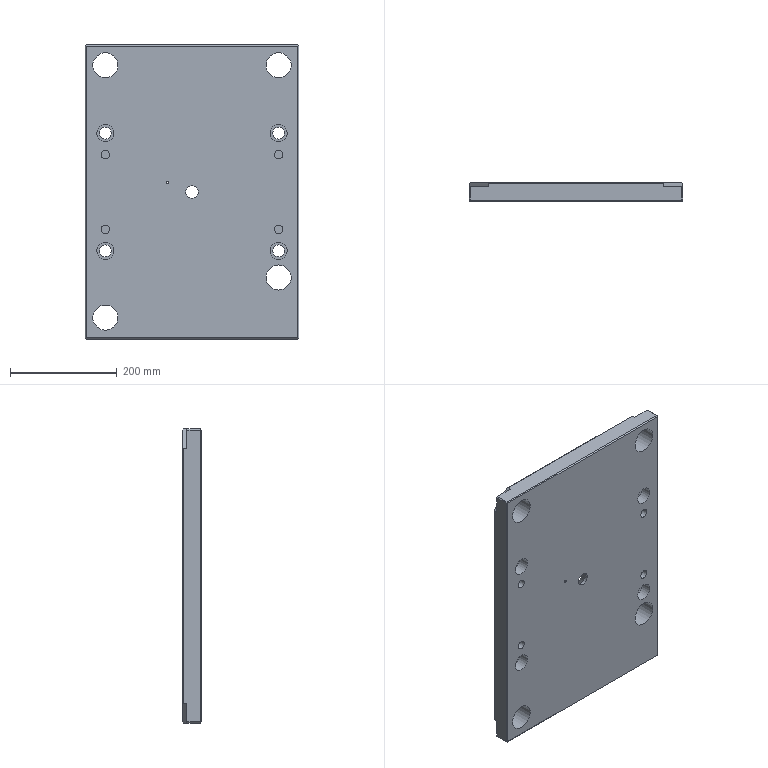Part | STEP file | SUPPORT-PLATE_id510_x_t | 1 solid | 53 faces | box 400 x 35 x 550 mm | volume 7237990 mm3 | plane 34 | cylinder 16 | cone 3 | commonest cylinder face diameters 16 x4 22 x4 32 x4 47 x4
STEP:
#1=CARTESIAN_POINT('',(-199.,91.5,-274.));
#2=VERTEX_POINT('',#1);
#3=CARTESIAN_POINT('',(-200.,92.5,-273.));
#4=VERTEX_POINT('',#3);
#5=CARTESIAN_POINT('',(-199.,91.5,-274.));
#6=DIRECTION('',(-0.5774,0.5774,0.5774));
#7=VECTOR('',#6,1.);
#8=LINE('',#5,#7);
#9=EDGE_CURVE('',#2,#4,#8,.T.);
#10=ORIENTED_EDGE('',*,*,#9,.T.);
#11=CARTESIAN_POINT('',(-200.,117.5,-273.));
#12=VERTEX_POINT('',#11);
#13=CARTESIAN_POINT('',(-200.,90.5,-273.));
#14=DIRECTION('',(0.,-1.,0.));
#15=VECTOR('',#14,1.);
#16=LINE('',#13,#15);
#17=EDGE_CURVE('',#12,#4,#16,.T.);
#18=ORIENTED_EDGE('',*,*,#17,.F.);
#19=CARTESIAN_POINT('',(-198.,117.5,-275.));
#20=VERTEX_POINT('',#19);
#21=CARTESIAN_POINT('',(-198.,117.5,-275.));
#22=DIRECTION('',(-0.7071,0.,0.7071));
#23=VECTOR('',#22,1.);
#24=LINE('',#21,#23);
#25=EDGE_CURVE('',#20,#12,#24,.T.);
#26=ORIENTED_EDGE('',*,*,#25,.F.);
#27=CARTESIAN_POINT('',(-198.,92.5,-275.));
#28=VERTEX_POINT('',#27);
#29=CARTESIAN_POINT('',(-198.,90.5,-275.));
#30=DIRECTION('',(0.,1.,0.));
#31=VECTOR('',#30,1.);
#32=LINE('',#29,#31);
#33=EDGE_CURVE('',#28,#20,#32,.T.);
#34=ORIENTED_EDGE('',*,*,#33,.F.);
#35=CARTESIAN_POINT('',(-198.,92.5,-275.));
#36=DIRECTION('',(-0.5774,-0.5774,0.5774));
#37=VECTOR('',#36,1.);
#38=LINE('',#35,#37);
#39=EDGE_CURVE('',#28,#2,#38,.T.);
#40=ORIENTED_EDGE('',*,*,#39,.T.);
#41=EDGE_LOOP('',(#10,#18,#26,#34,#40));
#42=FACE_OUTER_BOUND('',#41,.T.);
#43=CARTESIAN_POINT('',(-200.,92.5,-273.));
#44=DIRECTION('',(-0.7071,0.,-0.7071));
#45=DIRECTION('',(-0.7071,0.,0.7071));
#46=AXIS2_PLACEMENT_3D('',#43,#44,#45);
#47=PLANE('',#46);
#48=ADVANCED_FACE('',(#42),#47,.T.);
#49=CARTESIAN_POINT('',(-200.,117.5,-239.));
#50=VERTEX_POINT('',#49);
#51=CARTESIAN_POINT('',(-164.,117.5,-275.));
#52=VERTEX_POINT('',#51);
#53=CARTESIAN_POINT('',(-200.,117.5,-239.));
#54=DIRECTION('',(0.7071,0.,-0.7071));
#55=VECTOR('',#54,1.);
#56=LINE('',#53,#55);
#57=EDGE_CURVE('',#50,#52,#56,.T.);
#58=ORIENTED_EDGE('',*,*,#57,.T.);
#59=CARTESIAN_POINT('',(200.,117.5,-275.));
#60=DIRECTION('',(1.,0.,0.));
#61=VECTOR('',#60,1.);
#62=LINE('',#59,#61);
#63=EDGE_CURVE('',#20,#52,#62,.T.);
#64=ORIENTED_EDGE('',*,*,#63,.F.);
#65=ORIENTED_EDGE('',*,*,#25,.T.);
#66=CARTESIAN_POINT('',(-200.,117.5,-275.));
#67=DIRECTION('',(0.,0.,-1.));
#68=VECTOR('',#67,1.);
#69=LINE('',#66,#68);
#70=EDGE_CURVE('',#50,#12,#69,.T.);
#71=ORIENTED_EDGE('',*,*,#70,.F.);
#72=EDGE_LOOP('',(#58,#64,#65,#71));
#73=FACE_OUTER_BOUND('',#72,.T.);
#74=CARTESIAN_POINT('',(200.,117.5,-275.));
#75=DIRECTION('',(0.,1.,0.));
#76=DIRECTION('',(0.,0.,1.));
#77=AXIS2_PLACEMENT_3D('',#74,#75,#76);
#78=PLANE('',#77);
#79=ADVANCED_FACE('',(#73),#78,.T.);
#80=CARTESIAN_POINT('',(-199.,91.5,274.));
#81=VERTEX_POINT('',#80);
#82=CARTESIAN_POINT('',(-198.,92.5,275.));
#83=VERTEX_POINT('',#82);
#84=CARTESIAN_POINT('',(-199.,91.5,274.));
#85=DIRECTION('',(0.5774,0.5774,0.5774));
#86=VECTOR('',#85,1.);
#87=LINE('',#84,#86);
#88=EDGE_CURVE('',#81,#83,#87,.T.);
#89=ORIENTED_EDGE('',*,*,#88,.T.);
#90=CARTESIAN_POINT('',(-198.,117.5,275.));
#91=VERTEX_POINT('',#90);
#92=CARTESIAN_POINT('',(-198.,90.5,275.));
#93=DIRECTION('',(0.,-1.,0.));
#94=VECTOR('',#93,1.);
#95=LINE('',#92,#94);
#96=EDGE_CURVE('',#91,#83,#95,.T.);
#97=ORIENTED_EDGE('',*,*,#96,.F.);
#98=CARTESIAN_POINT('',(-200.,117.5,273.));
#99=VERTEX_POINT('',#98);
#100=CARTESIAN_POINT('',(-200.,117.5,273.));
#101=DIRECTION('',(0.7071,0.,0.7071));
#102=VECTOR('',#101,1.);
#103=LINE('',#100,#102);
#104=EDGE_CURVE('',#99,#91,#103,.T.);
#105=ORIENTED_EDGE('',*,*,#104,.F.);
#106=CARTESIAN_POINT('',(-200.,92.5,273.));
#107=VERTEX_POINT('',#106);
#108=CARTESIAN_POINT('',(-200.,90.5,273.));
#109=DIRECTION('',(0.,1.,0.));
#110=VECTOR('',#109,1.);
#111=LINE('',#108,#110);
#112=EDGE_CURVE('',#107,#99,#111,.T.);
#113=ORIENTED_EDGE('',*,*,#112,.F.);
#114=CARTESIAN_POINT('',(-200.,92.5,273.));
#115=DIRECTION('',(0.5774,-0.5774,0.5774));
#116=VECTOR('',#115,1.);
#117=LINE('',#114,#116);
#118=EDGE_CURVE('',#107,#81,#117,.T.);
#119=ORIENTED_EDGE('',*,*,#118,.T.);
#120=EDGE_LOOP('',(#89,#97,#105,#113,#119));
#121=FACE_OUTER_BOUND('',#120,.T.);
#122=CARTESIAN_POINT('',(-198.,90.5,275.));
#123=DIRECTION('',(-0.7071,0.,0.7071));
#124=DIRECTION('',(0.7071,0.,0.7071));
#125=AXIS2_PLACEMENT_3D('',#122,#123,#124);
#126=PLANE('',#125);
#127=ADVANCED_FACE('',(#121),#126,.T.);
#128=CARTESIAN_POINT('',(-164.,117.5,275.));
#129=VERTEX_POINT('',#128);
#130=CARTESIAN_POINT('',(-200.,117.5,239.));
#131=VERTEX_POINT('',#130);
#132=CARTESIAN_POINT('',(-164.,117.5,275.));
#133=DIRECTION('',(-0.7071,0.,-0.7071));
#134=VECTOR('',#133,1.);
#135=LINE('',#132,#134);
#136=EDGE_CURVE('',#129,#131,#135,.T.);
#137=ORIENTED_EDGE('',*,*,#136,.T.);
#138=CARTESIAN_POINT('',(-200.,117.5,-275.));
#139=DIRECTION('',(0.,0.,-1.));
#140=VECTOR('',#139,1.);
#141=LINE('',#138,#140);
#142=EDGE_CURVE('',#99,#131,#141,.T.);
#143=ORIENTED_EDGE('',*,*,#142,.F.);
#144=ORIENTED_EDGE('',*,*,#104,.T.);
#145=CARTESIAN_POINT('',(-200.,117.5,275.));
#146=DIRECTION('',(-1.,0.,0.));
#147=VECTOR('',#146,1.);
#148=LINE('',#145,#147);
#149=EDGE_CURVE('',#129,#91,#148,.T.);
#150=ORIENTED_EDGE('',*,*,#149,.F.);
#151=EDGE_LOOP('',(#137,#143,#144,#150));
#152=FACE_OUTER_BOUND('',#151,.T.);
#153=CARTESIAN_POINT('',(200.,117.5,-275.));
#154=DIRECTION('',(0.,1.,0.));
#155=DIRECTION('',(0.,0.,1.));
#156=AXIS2_PLACEMENT_3D('',#153,#154,#155);
#157=PLANE('',#156);
#158=ADVANCED_FACE('',(#152),#157,.T.);
#159=CARTESIAN_POINT('',(199.,91.5,274.));
#160=VERTEX_POINT('',#159);
#161=CARTESIAN_POINT('',(200.,92.5,273.));
#162=VERTEX_POINT('',#161);
#163=CARTESIAN_POINT('',(199.,91.5,274.));
#164=DIRECTION('',(0.5774,0.5774,-0.5774));
#165=VECTOR('',#164,1.);
#166=LINE('',#163,#165);
#167=EDGE_CURVE('',#160,#162,#166,.T.);
#168=ORIENTED_EDGE('',*,*,#167,.T.);
#169=CARTESIAN_POINT('',(200.,117.5,273.));
#170=VERTEX_POINT('',#169);
#171=CARTESIAN_POINT('',(200.,90.5,273.));
#172=DIRECTION('',(0.,-1.,0.));
#173=VECTOR('',#172,1.);
#174=LINE('',#171,#173);
#175=EDGE_CURVE('',#170,#162,#174,.T.);
#176=ORIENTED_EDGE('',*,*,#175,.F.);
#177=CARTESIAN_POINT('',(198.,117.5,275.));
#178=VERTEX_POINT('',#177);
#179=CARTESIAN_POINT('',(198.,117.5,275.));
#180=DIRECTION('',(0.7071,0.,-0.7071));
#181=VECTOR('',#180,1.);
#182=LINE('',#179,#181);
#183=EDGE_CURVE('',#178,#170,#182,.T.);
#184=ORIENTED_EDGE('',*,*,#183,.F.);
#185=CARTESIAN_POINT('',(198.,92.5,275.));
#186=VERTEX_POINT('',#185);
#187=CARTESIAN_POINT('',(198.,90.5,275.));
#188=DIRECTION('',(0.,1.,0.));
#189=VECTOR('',#188,1.);
#190=LINE('',#187,#189);
#191=EDGE_CURVE('',#186,#178,#190,.T.);
#192=ORIENTED_EDGE('',*,*,#191,.F.);
#193=CARTESIAN_POINT('',(198.,92.5,275.));
#194=DIRECTION('',(0.5774,-0.5774,-0.5774));
#195=VECTOR('',#194,1.);
#196=LINE('',#193,#195);
#197=EDGE_CURVE('',#186,#160,#196,.T.);
#198=ORIENTED_EDGE('',*,*,#197,.T.);
#199=EDGE_LOOP('',(#168,#176,#184,#192,#198));
#200=FACE_OUTER_BOUND('',#199,.T.);
#201=CARTESIAN_POINT('',(200.,90.5,273.));
#202=DIRECTION('',(0.7071,0.,0.7071));
#203=DIRECTION('',(0.7071,0.,-0.7071));
#204=AXIS2_PLACEMENT_3D('',#201,#202,#203);
#205=PLANE('',#204);
#206=ADVANCED_FACE('',(#200),#205,.T.);
#207=CARTESIAN_POINT('',(199.,91.5,-274.));
#208=VERTEX_POINT('',#207);
#209=CARTESIAN_POINT('',(198.,92.5,-275.));
#210=VERTEX_POINT('',#209);
#211=CARTESIAN_POINT('',(199.,91.5,-274.));
#212=DIRECTION('',(-0.5774,0.5774,-0.5774));
#213=VECTOR('',#212,1.);
#214=LINE('',#211,#213);
#215=EDGE_CURVE('',#208,#210,#214,.T.);
#216=ORIENTED_EDGE('',*,*,#215,.T.);
#217=CARTESIAN_POINT('',(198.,117.5,-275.));
#218=VERTEX_POINT('',#217);
#219=CARTESIAN_POINT('',(198.,90.5,-275.));
#220=DIRECTION('',(0.,-1.,0.));
#221=VECTOR('',#220,1.);
#222=LINE('',#219,#221);
#223=EDGE_CURVE('',#218,#210,#222,.T.);
#224=ORIENTED_EDGE('',*,*,#223,.F.);
#225=CARTESIAN_POINT('',(200.,117.5,-273.));
#226=VERTEX_POINT('',#225);
#227=CARTESIAN_POINT('',(200.,117.5,-273.));
#228=DIRECTION('',(-0.7071,0.,-0.7071));
#229=VECTOR('',#228,1.);
#230=LINE('',#227,#229);
#231=EDGE_CURVE('',#226,#218,#230,.T.);
#232=ORIENTED_EDGE('',*,*,#231,.F.);
#233=CARTESIAN_POINT('',(200.,92.5,-273.));
#234=VERTEX_POINT('',#233);
#235=CARTESIAN_POINT('',(200.,90.5,-273.));
#236=DIRECTION('',(0.,1.,0.));
#237=VECTOR('',#236,1.);
#238=LINE('',#235,#237);
#239=EDGE_CURVE('',#234,#226,#238,.T.);
#240=ORIENTED_EDGE('',*,*,#239,.F.);
#241=CARTESIAN_POINT('',(200.,92.5,-273.));
#242=DIRECTION('',(-0.5774,-0.5774,-0.5774));
#243=VECTOR('',#242,1.);
#244=LINE('',#241,#243);
#245=EDGE_CURVE('',#234,#208,#244,.T.);
#246=ORIENTED_EDGE('',*,*,#245,.T.);
#247=EDGE_LOOP('',(#216,#224,#232,#240,#246));
#248=FACE_OUTER_BOUND('',#247,.T.);
#249=CARTESIAN_POINT('',(198.,90.5,-275.));
#250=DIRECTION('',(0.7071,0.,-0.7071));
#251=DIRECTION('',(-0.7071,0.,-0.7071));
#252=AXIS2_PLACEMENT_3D('',#249,#250,#251);
#253=PLANE('',#252);
#254=ADVANCED_FACE('',(#248),#253,.T.);
#255=ORIENTED_EDGE('',*,*,#231,.T.);
#256=CARTESIAN_POINT('',(164.,117.5,-275.));
#257=VERTEX_POINT('',#256);
#258=CARTESIAN_POINT('',(200.,117.5,-275.));
#259=DIRECTION('',(1.,0.,0.));
#260=VECTOR('',#259,1.);
#261=LINE('',#258,#260);
#262=EDGE_CURVE('',#257,#218,#261,.T.);
#263=ORIENTED_EDGE('',*,*,#262,.F.);
#264=CARTESIAN_POINT('',(200.,117.5,-239.));
#265=VERTEX_POINT('',#264);
#266=CARTESIAN_POINT('',(164.,117.5,-275.));
#267=DIRECTION('',(0.7071,0.,0.7071));
#268=VECTOR('',#267,1.);
#269=LINE('',#266,#268);
#270=EDGE_CURVE('',#257,#265,#269,.T.);
#271=ORIENTED_EDGE('',*,*,#270,.T.);
#272=CARTESIAN_POINT('',(200.,117.5,275.));
#273=DIRECTION('',(0.,0.,1.));
#274=VECTOR('',#273,1.);
#275=LINE('',#272,#274);
#276=EDGE_CURVE('',#226,#265,#275,.T.);
#277=ORIENTED_EDGE('',*,*,#276,.F.);
#278=EDGE_LOOP('',(#255,#263,#271,#277));
#279=FACE_OUTER_BOUND('',#278,.T.);
#280=CARTESIAN_POINT('',(200.,117.5,-275.));
#281=DIRECTION('',(0.,1.,0.));
#282=DIRECTION('',(0.,0.,1.));
#283=AXIS2_PLACEMENT_3D('',#280,#281,#282);
#284=PLANE('',#283);
#285=ADVANCED_FACE('',(#279),#284,.T.);
#286=CARTESIAN_POINT('',(200.,117.5,239.));
#287=VERTEX_POINT('',#286);
#288=CARTESIAN_POINT('',(164.,117.5,275.));
#289=VERTEX_POINT('',#288);
#290=CARTESIAN_POINT('',(200.,117.5,239.));
#291=DIRECTION('',(-0.7071,0.,0.7071));
#292=VECTOR('',#291,1.);
#293=LINE('',#290,#292);
#294=EDGE_CURVE('',#287,#289,#293,.T.);
#295=ORIENTED_EDGE('',*,*,#294,.T.);
#296=CARTESIAN_POINT('',(-200.,117.5,275.));
#297=DIRECTION('',(-1.,0.,0.));
#298=VECTOR('',#297,1.);
#299=LINE('',#296,#298);
#300=EDGE_CURVE('',#178,#289,#299,.T.);
#301=ORIENTED_EDGE('',*,*,#300,.F.);
#302=ORIENTED_EDGE('',*,*,#183,.T.);
#303=CARTESIAN_POINT('',(200.,117.5,275.));
#304=DIRECTION('',(0.,0.,1.));
#305=VECTOR('',#304,1.);
#306=LINE('',#303,#305);
#307=EDGE_CURVE('',#287,#170,#306,.T.);
#308=ORIENTED_EDGE('',*,*,#307,.F.);
#309=EDGE_LOOP('',(#295,#301,#302,#308));
#310=FACE_OUTER_BOUND('',#309,.T.);
#311=CARTESIAN_POINT('',(200.,117.5,-275.));
#312=DIRECTION('',(0.,1.,0.));
#313=DIRECTION('',(0.,0.,1.));
#314=AXIS2_PLACEMENT_3D('',#311,#312,#313);
#315=PLANE('',#314);
#316=ADVANCED_FACE('',(#310),#315,.T.);
#317=CARTESIAN_POINT('',(-164.,123.5,-275.));
#318=VERTEX_POINT('',#317);
#319=CARTESIAN_POINT('',(164.,123.5,-275.));
#320=VERTEX_POINT('',#319);
#321=CARTESIAN_POINT('',(200.,123.5,-275.));
#322=DIRECTION('',(1.,0.,0.));
#323=VECTOR('',#322,1.);
#324=LINE('',#321,#323);
#325=EDGE_CURVE('',#318,#320,#324,.T.);
#326=ORIENTED_EDGE('',*,*,#325,.F.);
#327=CARTESIAN_POINT('',(-166.,125.5,-273.));
#328=VERTEX_POINT('',#327);
#329=CARTESIAN_POINT('',(-164.,123.5,-275.));
#330=DIRECTION('',(-0.5774,0.5774,0.5774));
#331=VECTOR('',#330,1.);
#332=LINE('',#329,#331);
#333=EDGE_CURVE('',#318,#328,#332,.T.);
#334=ORIENTED_EDGE('',*,*,#333,.T.);
#335=CARTESIAN_POINT('',(166.,125.5,-273.));
#336=VERTEX_POINT('',#335);
#337=CARTESIAN_POINT('',(-83.002,125.5,-273.));
#338=DIRECTION('',(-1.,0.,0.));
#339=VECTOR('',#338,1.);
#340=LINE('',#337,#339);
#341=EDGE_CURVE('',#336,#328,#340,.T.);
#342=ORIENTED_EDGE('',*,*,#341,.F.);
#343=CARTESIAN_POINT('',(166.,125.5,-273.));
#344=DIRECTION('',(-0.5774,-0.5774,-0.5774));
#345=VECTOR('',#344,1.);
#346=LINE('',#343,#345);
#347=EDGE_CURVE('',#336,#320,#346,.T.);
#348=ORIENTED_EDGE('',*,*,#347,.T.);
#349=EDGE_LOOP('',(#326,#334,#342,#348));
#350=FACE_OUTER_BOUND('',#349,.T.);
#351=CARTESIAN_POINT('',(166.,125.5,-273.));
#352=DIRECTION('',(0.,-0.7071,0.7071));
#353=DIRECTION('',(0.,-0.7071,-0.7071));
#354=AXIS2_PLACEMENT_3D('',#351,#352,#353);
#355=PLANE('',#354);
#356=ADVANCED_FACE('',(#350),#355,.F.);
#357=CARTESIAN_POINT('',(-164.,90.5,-275.));
#358=DIRECTION('',(0.,1.,0.));
#359=VECTOR('',#358,1.);
#360=LINE('',#357,#359);
#361=EDGE_CURVE('',#52,#318,#360,.T.);
#362=ORIENTED_EDGE('',*,*,#361,.F.);
#363=ORIENTED_EDGE('',*,*,#57,.F.);
#364=CARTESIAN_POINT('',(-200.,123.5,-239.));
#365=VERTEX_POINT('',#364);
#366=CARTESIAN_POINT('',(-200.,90.5,-239.));
#367=DIRECTION('',(0.,-1.,0.));
#368=VECTOR('',#367,1.);
#369=LINE('',#366,#368);
#370=EDGE_CURVE('',#365,#50,#369,.T.);
#371=ORIENTED_EDGE('',*,*,#370,.F.);
#372=CARTESIAN_POINT('',(-198.,125.5,-241.));
#373=VERTEX_POINT('',#372);
#374=CARTESIAN_POINT('',(-200.,123.5,-239.));
#375=DIRECTION('',(0.5774,0.5774,-0.5774));
#376=VECTOR('',#375,1.);
#377=LINE('',#374,#376);
#378=EDGE_CURVE('',#365,#373,#377,.T.);
#379=ORIENTED_EDGE('',*,*,#378,.T.);
#380=CARTESIAN_POINT('',(-166.,125.5,-273.));
#381=DIRECTION('',(-0.7071,0.,0.7071));
#382=VECTOR('',#381,1.);
#383=LINE('',#380,#382);
#384=EDGE_CURVE('',#328,#373,#383,.T.);
#385=ORIENTED_EDGE('',*,*,#384,.F.);
#386=ORIENTED_EDGE('',*,*,#333,.F.);
#387=EDGE_LOOP('',(#362,#363,#371,#379,#385,#386));
#388=FACE_OUTER_BOUND('',#387,.T.);
#389=CARTESIAN_POINT('',(-200.,125.5,-239.));
#390=DIRECTION('',(0.7071,0.,0.7071));
#391=DIRECTION('',(0.7071,0.,-0.7071));
#392=AXIS2_PLACEMENT_3D('',#389,#390,#391);
#393=PLANE('',#392);
#394=ADVANCED_FACE('',(#388),#393,.F.);
#395=CARTESIAN_POINT('',(-200.,123.5,239.));
#396=VERTEX_POINT('',#395);
#397=CARTESIAN_POINT('',(-200.,123.5,-275.));
#398=DIRECTION('',(0.,0.,-1.));
#399=VECTOR('',#398,1.);
#400=LINE('',#397,#399);
#401=EDGE_CURVE('',#396,#365,#400,.T.);
#402=ORIENTED_EDGE('',*,*,#401,.F.);
#403=CARTESIAN_POINT('',(-198.,125.5,241.));
#404=VERTEX_POINT('',#403);
#405=CARTESIAN_POINT('',(-200.,123.5,239.));
#406=DIRECTION('',(0.5774,0.5774,0.5774));
#407=VECTOR('',#406,1.);
#408=LINE('',#405,#407);
#409=EDGE_CURVE('',#396,#404,#408,.T.);
#410=ORIENTED_EDGE('',*,*,#409,.T.);
#411=CARTESIAN_POINT('',(-198.,125.5,-70.535));
#412=DIRECTION('',(0.,0.,1.));
#413=VECTOR('',#412,1.);
#414=LINE('',#411,#413);
#415=EDGE_CURVE('',#373,#404,#414,.T.);
#416=ORIENTED_EDGE('',*,*,#415,.F.);
#417=ORIENTED_EDGE('',*,*,#378,.F.);
#418=EDGE_LOOP('',(#402,#410,#416,#417));
#419=FACE_OUTER_BOUND('',#418,.T.);
#420=CARTESIAN_POINT('',(-198.,125.5,-241.));
#421=DIRECTION('',(0.7071,-0.7071,0.));
#422=DIRECTION('',(0.7071,0.7071,0.));
#423=AXIS2_PLACEMENT_3D('',#420,#421,#422);
#424=PLANE('',#423);
#425=ADVANCED_FACE('',(#419),#424,.F.);
#426=CARTESIAN_POINT('',(-200.,90.5,239.));
#427=DIRECTION('',(0.,1.,0.));
#428=VECTOR('',#427,1.);
#429=LINE('',#426,#428);
#430=EDGE_CURVE('',#131,#396,#429,.T.);
#431=ORIENTED_EDGE('',*,*,#430,.F.);
#432=ORIENTED_EDGE('',*,*,#136,.F.);
#433=CARTESIAN_POINT('',(-164.,123.5,275.));
#434=VERTEX_POINT('',#433);
#435=CARTESIAN_POINT('',(-164.,90.5,275.));
#436=DIRECTION('',(0.,-1.,0.));
#437=VECTOR('',#436,1.);
#438=LINE('',#435,#437);
#439=EDGE_CURVE('',#434,#129,#438,.T.);
#440=ORIENTED_EDGE('',*,*,#439,.F.);
#441=CARTESIAN_POINT('',(-166.,125.5,273.));
#442=VERTEX_POINT('',#441);
#443=CARTESIAN_POINT('',(-164.,123.5,275.));
#444=DIRECTION('',(-0.5774,0.5774,-0.5774));
#445=VECTOR('',#444,1.);
#446=LINE('',#443,#445);
#447=EDGE_CURVE('',#434,#442,#446,.T.);
#448=ORIENTED_EDGE('',*,*,#447,.T.);
#449=CARTESIAN_POINT('',(-198.,125.5,241.));
#450=DIRECTION('',(0.7071,0.,0.7071));
#451=VECTOR('',#450,1.);
#452=LINE('',#449,#451);
#453=EDGE_CURVE('',#404,#442,#452,.T.);
#454=ORIENTED_EDGE('',*,*,#453,.F.);
#455=ORIENTED_EDGE('',*,*,#409,.F.);
#456=EDGE_LOOP('',(#431,#432,#440,#448,#454,#455));
#457=FACE_OUTER_BOUND('',#456,.T.);
#458=CARTESIAN_POINT('',(-164.,125.5,275.));
#459=DIRECTION('',(0.7071,0.,-0.7071));
#460=DIRECTION('',(-0.7071,0.,-0.7071));
#461=AXIS2_PLACEMENT_3D('',#458,#459,#460);
#462=PLANE('',#461);
#463=ADVANCED_FACE('',(#457),#462,.F.);
#464=CARTESIAN_POINT('',(164.,123.5,275.));
#465=VERTEX_POINT('',#464);
#466=CARTESIAN_POINT('',(-200.,123.5,275.));
#467=DIRECTION('',(-1.,0.,0.));
#468=VECTOR('',#467,1.);
#469=LINE('',#466,#468);
#470=EDGE_CURVE('',#465,#434,#469,.T.);
#471=ORIENTED_EDGE('',*,*,#470,.F.);
#472=CARTESIAN_POINT('',(166.,125.5,273.));
#473=VERTEX_POINT('',#472);
#474=CARTESIAN_POINT('',(164.,123.5,275.));
#475=DIRECTION('',(0.5774,0.5774,-0.5774));
#476=VECTOR('',#475,1.);
#477=LINE('',#474,#476);
#478=EDGE_CURVE('',#465,#473,#477,.T.);
#479=ORIENTED_EDGE('',*,*,#478,.T.);
#480=CARTESIAN_POINT('',(-83.002,125.5,273.));
#481=DIRECTION('',(1.,0.,0.));
#482=VECTOR('',#481,1.);
#483=LINE('',#480,#482);
#484=EDGE_CURVE('',#442,#473,#483,.T.);
#485=ORIENTED_EDGE('',*,*,#484,.F.);
#486=ORIENTED_EDGE('',*,*,#447,.F.);
#487=EDGE_LOOP('',(#471,#479,#485,#486));
#488=FACE_OUTER_BOUND('',#487,.T.);
#489=CARTESIAN_POINT('',(-166.,125.5,273.));
#490=DIRECTION('',(0.,-0.7071,-0.7071));
#491=DIRECTION('',(0.,0.7071,-0.7071));
#492=AXIS2_PLACEMENT_3D('',#489,#490,#491);
#493=PLANE('',#492);
#494=ADVANCED_FACE('',(#488),#493,.F.);
#495=CARTESIAN_POINT('',(164.,90.5,275.));
#496=DIRECTION('',(0.,1.,0.));
#497=VECTOR('',#496,1.);
#498=LINE('',#495,#497);
#499=EDGE_CURVE('',#289,#465,#498,.T.);
#500=ORIENTED_EDGE('',*,*,#499,.F.);
#501=ORIENTED_EDGE('',*,*,#294,.F.);
#502=CARTESIAN_POINT('',(200.,123.5,239.));
#503=VERTEX_POINT('',#502);
#504=CARTESIAN_POINT('',(200.,90.5,239.));
#505=DIRECTION('',(0.,-1.,0.));
#506=VECTOR('',#505,1.);
#507=LINE('',#504,#506);
#508=EDGE_CURVE('',#503,#287,#507,.T.);
#509=ORIENTED_EDGE('',*,*,#508,.F.);
#510=CARTESIAN_POINT('',(198.,125.5,241.));
#511=VERTEX_POINT('',#510);
#512=CARTESIAN_POINT('',(200.,123.5,239.));
#513=DIRECTION('',(-0.5774,0.5774,0.5774));
#514=VECTOR('',#513,1.);
#515=LINE('',#512,#514);
#516=EDGE_CURVE('',#503,#511,#515,.T.);
#517=ORIENTED_EDGE('',*,*,#516,.T.);
#518=CARTESIAN_POINT('',(166.,125.5,273.));
#519=DIRECTION('',(0.7071,0.,-0.7071));
#520=VECTOR('',#519,1.);
#521=LINE('',#518,#520);
#522=EDGE_CURVE('',#473,#511,#521,.T.);
#523=ORIENTED_EDGE('',*,*,#522,.F.);
#524=ORIENTED_EDGE('',*,*,#478,.F.);
#525=EDGE_LOOP('',(#500,#501,#509,#517,#523,#524));
#526=FACE_OUTER_BOUND('',#525,.T.);
#527=CARTESIAN_POINT('',(200.,125.5,239.));
#528=DIRECTION('',(-0.7071,0.,-0.7071));
#529=DIRECTION('',(-0.7071,0.,0.7071));
#530=AXIS2_PLACEMENT_3D('',#527,#528,#529);
#531=PLANE('',#530);
#532=ADVANCED_FACE('',(#526),#531,.F.);
#533=CARTESIAN_POINT('',(200.,123.5,-239.));
#534=VERTEX_POINT('',#533);
#535=CARTESIAN_POINT('',(200.,123.5,275.));
#536=DIRECTION('',(0.,0.,1.));
#537=VECTOR('',#536,1.);
#538=LINE('',#535,#537);
#539=EDGE_CURVE('',#534,#503,#538,.T.);
#540=ORIENTED_EDGE('',*,*,#539,.F.);
#541=CARTESIAN_POINT('',(198.,125.5,-241.));
#542=VERTEX_POINT('',#541);
#543=CARTESIAN_POINT('',(200.,123.5,-239.));
#544=DIRECTION('',(-0.5774,0.5774,-0.5774));
#545=VECTOR('',#544,1.);
#546=LINE('',#543,#545);
#547=EDGE_CURVE('',#534,#542,#546,.T.);
#548=ORIENTED_EDGE('',*,*,#547,.T.);
#549=CARTESIAN_POINT('',(198.,125.5,-70.535));
#550=DIRECTION('',(0.,0.,-1.));
#551=VECTOR('',#550,1.);
#552=LINE('',#549,#551);
#553=EDGE_CURVE('',#511,#542,#552,.T.);
#554=ORIENTED_EDGE('',*,*,#553,.F.);
#555=ORIENTED_EDGE('',*,*,#516,.F.);
#556=EDGE_LOOP('',(#540,#548,#554,#555));
#557=FACE_OUTER_BOUND('',#556,.T.);
#558=CARTESIAN_POINT('',(198.,125.5,241.));
#559=DIRECTION('',(-0.7071,-0.7071,0.));
#560=DIRECTION('',(0.7071,-0.7071,0.));
#561=AXIS2_PLACEMENT_3D('',#558,#559,#560);
#562=PLANE('',#561);
#563=ADVANCED_FACE('',(#557),#562,.F.);
#564=CARTESIAN_POINT('',(200.,90.5,-239.));
#565=DIRECTION('',(0.,1.,0.));
#566=VECTOR('',#565,1.);
#567=LINE('',#564,#566);
#568=EDGE_CURVE('',#265,#534,#567,.T.);
#569=ORIENTED_EDGE('',*,*,#568,.F.);
#570=ORIENTED_EDGE('',*,*,#270,.F.);
#571=CARTESIAN_POINT('',(164.,90.5,-275.));
#572=DIRECTION('',(0.,-1.,0.));
#573=VECTOR('',#572,1.);
#574=LINE('',#571,#573);
#575=EDGE_CURVE('',#320,#257,#574,.T.);
#576=ORIENTED_EDGE('',*,*,#575,.F.);
#577=ORIENTED_EDGE('',*,*,#347,.F.);
#578=CARTESIAN_POINT('',(198.,125.5,-241.));
#579=DIRECTION('',(-0.7071,0.,-0.7071));
#580=VECTOR('',#579,1.);
#581=LINE('',#578,#580);
#582=EDGE_CURVE('',#542,#336,#581,.T.);
#583=ORIENTED_EDGE('',*,*,#582,.F.);
#584=ORIENTED_EDGE('',*,*,#547,.F.);
#585=EDGE_LOOP('',(#569,#570,#576,#577,#583,#584));
#586=FACE_OUTER_BOUND('',#585,.T.);
#587=CARTESIAN_POINT('',(164.,125.5,-275.));
#588=DIRECTION('',(-0.7071,0.,0.7071));
#589=DIRECTION('',(0.7071,0.,0.7071));
#590=AXIS2_PLACEMENT_3D('',#587,#588,#589);
#591=PLANE('',#590);
#592=ADVANCED_FACE('',(#586),#591,.F.);
#593=CARTESIAN_POINT('',(-162.,125.5,-121.));
#594=VERTEX_POINT('',#593);
#595=CARTESIAN_POINT('',(-162.,125.5,-110.));
#596=DIRECTION('',(0.,-1.,0.));
#597=DIRECTION('',(0.,0.,-1.));
#598=AXIS2_PLACEMENT_3D('',#595,#596,#597);
#599=CIRCLE('',#598,11.);
#600=EDGE_CURVE('',#594,#594,#599,.T.);
#601=ORIENTED_EDGE('',*,*,#600,.F.);
#602=EDGE_LOOP('',(#601));
#603=FACE_BOUND('',#602,.T.);
#604=CARTESIAN_POINT('',(-162.,110.5,-121.));
#605=VERTEX_POINT('',#604);
#606=CARTESIAN_POINT('',(-162.,110.5,-110.));
#607=DIRECTION('',(0.,1.,0.));
#608=DIRECTION('',(0.,0.,-1.));
#609=AXIS2_PLACEMENT_3D('',#606,#607,#608);
#610=CIRCLE('',#609,11.);
#611=EDGE_CURVE('',#605,#605,#610,.T.);
#612=ORIENTED_EDGE('',*,*,#611,.F.);
#613=EDGE_LOOP('',(#612));
#614=FACE_BOUND('',#613,.T.);
#615=CARTESIAN_POINT('',(-162.,90.5,-110.));
#616=DIRECTION('',(0.,-1.,0.));
#617=DIRECTION('',(0.,0.,-1.));
#618=AXIS2_PLACEMENT_3D('',#615,#616,#617);
#619=CYLINDRICAL_SURFACE('',#618,11.);
#620=ADVANCED_FACE('',(#603,#614),#619,.F.);
#621=CARTESIAN_POINT('',(162.,125.5,-121.));
#622=VERTEX_POINT('',#621);
#623=CARTESIAN_POINT('',(162.,125.5,-110.));
#624=DIRECTION('',(0.,-1.,0.));
#625=DIRECTION('',(0.,0.,-1.));
#626=AXIS2_PLACEMENT_3D('',#623,#624,#625);
#627=CIRCLE('',#626,11.);
#628=EDGE_CURVE('',#622,#622,#627,.T.);
#629=ORIENTED_EDGE('',*,*,#628,.F.);
#630=EDGE_LOOP('',(#629));
#631=FACE_BOUND('',#630,.T.);
#632=CARTESIAN_POINT('',(162.,110.5,-121.));
#633=VERTEX_POINT('',#632);
#634=CARTESIAN_POINT('',(162.,110.5,-110.));
#635=DIRECTION('',(0.,1.,0.));
#636=DIRECTION('',(0.,0.,-1.));
#637=AXIS2_PLACEMENT_3D('',#634,#635,#636);
#638=CIRCLE('',#637,11.);
#639=EDGE_CURVE('',#633,#633,#638,.T.);
#640=ORIENTED_EDGE('',*,*,#639,.F.);
#641=EDGE_LOOP('',(#640));
#642=FACE_BOUND('',#641,.T.);
#643=CARTESIAN_POINT('',(162.,90.5,-110.));
#644=DIRECTION('',(0.,-1.,0.));
#645=DIRECTION('',(0.,0.,-1.));
#646=AXIS2_PLACEMENT_3D('',#643,#644,#645);
#647=CYLINDRICAL_SURFACE('',#646,11.);
#648=ADVANCED_FACE('',(#631,#642),#647,.F.);
#649=CARTESIAN_POINT('',(162.,125.5,99.));
#650=VERTEX_POINT('',#649);
#651=CARTESIAN_POINT('',(162.,125.5,110.));
#652=DIRECTION('',(0.,-1.,0.));
#653=DIRECTION('',(0.,0.,-1.));
#654=AXIS2_PLACEMENT_3D('',#651,#652,#653);
#655=CIRCLE('',#654,11.);
#656=EDGE_CURVE('',#650,#650,#655,.T.);
#657=ORIENTED_EDGE('',*,*,#656,.F.);
#658=EDGE_LOOP('',(#657));
#659=FACE_BOUND('',#658,.T.);
#660=CARTESIAN_POINT('',(162.,110.5,99.));
#661=VERTEX_POINT('',#660);
#662=CARTESIAN_POINT('',(162.,110.5,110.));
#663=DIRECTION('',(0.,1.,0.));
#664=DIRECTION('',(0.,0.,-1.));
#665=AXIS2_PLACEMENT_3D('',#662,#663,#664);
#666=CIRCLE('',#665,11.);
#667=EDGE_CURVE('',#661,#661,#666,.T.);
#668=ORIENTED_EDGE('',*,*,#667,.F.);
#669=EDGE_LOOP('',(#668));
#670=FACE_BOUND('',#669,.T.);
#671=CARTESIAN_POINT('',(162.,90.5,110.));
#672=DIRECTION('',(0.,-1.,0.));
#673=DIRECTION('',(0.,0.,-1.));
#674=AXIS2_PLACEMENT_3D('',#671,#672,#673);
#675=CYLINDRICAL_SURFACE('',#674,11.);
#676=ADVANCED_FACE('',(#659,#670),#675,.F.);
#677=CARTESIAN_POINT('',(-162.,125.5,99.));
#678=VERTEX_POINT('',#677);
#679=CARTESIAN_POINT('',(-162.,125.5,110.));
#680=DIRECTION('',(0.,-1.,0.));
#681=DIRECTION('',(0.,0.,-1.));
#682=AXIS2_PLACEMENT_3D('',#679,#680,#681);
#683=CIRCLE('',#682,11.);
#684=EDGE_CURVE('',#678,#678,#683,.T.);
#685=ORIENTED_EDGE('',*,*,#684,.F.);
#686=EDGE_LOOP('',(#685));
#687=FACE_BOUND('',#686,.T.);
#688=CARTESIAN_POINT('',(-162.,110.5,99.));
#689=VERTEX_POINT('',#688);
#690=CARTESIAN_POINT('',(-162.,110.5,110.));
#691=DIRECTION('',(0.,1.,0.));
#692=DIRECTION('',(0.,0.,-1.));
#693=AXIS2_PLACEMENT_3D('',#690,#691,#692);
#694=CIRCLE('',#693,11.);
#695=EDGE_CURVE('',#689,#689,#694,.T.);
#696=ORIENTED_EDGE('',*,*,#695,.F.);
#697=EDGE_LOOP('',(#696));
#698=FACE_BOUND('',#697,.T.);
#699=CARTESIAN_POINT('',(-162.,90.5,110.));
#700=DIRECTION('',(0.,-1.,0.));
#701=DIRECTION('',(0.,0.,-1.));
#702=AXIS2_PLACEMENT_3D('',#699,#700,#701);
#703=CYLINDRICAL_SURFACE('',#702,11.);
#704=ADVANCED_FACE('',(#687,#698),#703,.F.);
#705=ORIENTED_EDGE('',*,*,#575,.T.);
#706=ORIENTED_EDGE('',*,*,#262,.T.);
#707=ORIENTED_EDGE('',*,*,#223,.T.);
#708=CARTESIAN_POINT('',(198.,92.5,-275.));
#709=DIRECTION('',(1.,0.,0.));
#710=VECTOR('',#709,1.);
#711=LINE('',#708,#710);
#712=EDGE_CURVE('',#28,#210,#711,.T.);
#713=ORIENTED_EDGE('',*,*,#712,.F.);
#714=ORIENTED_EDGE('',*,*,#33,.T.);
#715=ORIENTED_EDGE('',*,*,#63,.T.);
#716=ORIENTED_EDGE('',*,*,#361,.T.);
#717=ORIENTED_EDGE('',*,*,#325,.T.);
#718=EDGE_LOOP('',(#705,#706,#707,#713,#714,#715,#716,#717));
#719=FACE_OUTER_BOUND('',#718,.T.);
#720=CARTESIAN_POINT('',(200.,90.5,-275.));
#721=DIRECTION('',(0.,0.,-1.));
#722=DIRECTION('',(-1.,0.,0.));
#723=AXIS2_PLACEMENT_3D('',#720,#721,#722);
#724=PLANE('',#723);
#725=ADVANCED_FACE('',(#719),#724,.T.);
#726=ORIENTED_EDGE('',*,*,#370,.T.);
#727=ORIENTED_EDGE('',*,*,#70,.T.);
#728=ORIENTED_EDGE('',*,*,#17,.T.);
#729=CARTESIAN_POINT('',(-200.,92.5,-275.));
#730=DIRECTION('',(0.,0.,-1.));
#731=VECTOR('',#730,1.);
#732=LINE('',#729,#731);
#733=EDGE_CURVE('',#107,#4,#732,.T.);
#734=ORIENTED_EDGE('',*,*,#733,.F.);
#735=ORIENTED_EDGE('',*,*,#112,.T.);
#736=ORIENTED_EDGE('',*,*,#142,.T.);
#737=ORIENTED_EDGE('',*,*,#430,.T.);
#738=ORIENTED_EDGE('',*,*,#401,.T.);
#739=EDGE_LOOP('',(#726,#727,#728,#734,#735,#736,#737,#738));
#740=FACE_OUTER_BOUND('',#739,.T.);
#741=CARTESIAN_POINT('',(-200.,90.5,-275.));
#742=DIRECTION('',(-1.,0.,0.));
#743=DIRECTION('',(0.,0.,1.));
#744=AXIS2_PLACEMENT_3D('',#741,#742,#743);
#745=PLANE('',#744);
#746=ADVANCED_FACE('',(#740),#745,.T.);
#747=ORIENTED_EDGE('',*,*,#439,.T.);
#748=ORIENTED_EDGE('',*,*,#149,.T.);
#749=ORIENTED_EDGE('',*,*,#96,.T.);
#750=CARTESIAN_POINT('',(-200.,92.5,275.));
#751=DIRECTION('',(-1.,0.,0.));
#752=VECTOR('',#751,1.);
#753=LINE('',#750,#752);
#754=EDGE_CURVE('',#186,#83,#753,.T.);
#755=ORIENTED_EDGE('',*,*,#754,.F.);
#756=ORIENTED_EDGE('',*,*,#191,.T.);
#757=ORIENTED_EDGE('',*,*,#300,.T.);
#758=ORIENTED_EDGE('',*,*,#499,.T.);
#759=ORIENTED_EDGE('',*,*,#470,.T.);
#760=EDGE_LOOP('',(#747,#748,#749,#755,#756,#757,#758,#759));
#761=FACE_OUTER_BOUND('',#760,.T.);
#762=CARTESIAN_POINT('',(-200.,90.5,275.));
#763=DIRECTION('',(0.,0.,1.));
#764=DIRECTION('',(1.,0.,0.));
#765=AXIS2_PLACEMENT_3D('',#762,#763,#764);
#766=PLANE('',#765);
#767=ADVANCED_FACE('',(#761),#766,.T.);
#768=ORIENTED_EDGE('',*,*,#508,.T.);
#769=ORIENTED_EDGE('',*,*,#307,.T.);
#770=ORIENTED_EDGE('',*,*,#175,.T.);
#771=CARTESIAN_POINT('',(200.,92.5,273.));
#772=DIRECTION('',(0.,0.,1.));
#773=VECTOR('',#772,1.);
#774=LINE('',#771,#773);
#775=EDGE_CURVE('',#234,#162,#774,.T.);
#776=ORIENTED_EDGE('',*,*,#775,.F.);
#777=ORIENTED_EDGE('',*,*,#239,.T.);
#778=ORIENTED_EDGE('',*,*,#276,.T.);
#779=ORIENTED_EDGE('',*,*,#568,.T.);
#780=ORIENTED_EDGE('',*,*,#539,.T.);
#781=EDGE_LOOP('',(#768,#769,#770,#776,#777,#778,#779,#780));
#782=FACE_OUTER_BOUND('',#781,.T.);
#783=CARTESIAN_POINT('',(200.,90.5,275.));
#784=DIRECTION('',(1.,0.,0.));
#785=DIRECTION('',(0.,0.,-1.));
#786=AXIS2_PLACEMENT_3D('',#783,#784,#785);
#787=PLANE('',#786);
#788=ADVANCED_FACE('',(#782),#787,.T.);
#789=CARTESIAN_POINT('',(162.,115.5,-78.));
#790=VERTEX_POINT('',#789);
#791=CARTESIAN_POINT('',(162.,115.5,-70.));
#792=DIRECTION('',(0.,-1.,0.));
#793=DIRECTION('',(0.,0.,-1.));
#794=AXIS2_PLACEMENT_3D('',#791,#792,#793);
#795=CIRCLE('',#794,8.);
#796=EDGE_CURVE('',#790,#790,#795,.T.);
#797=ORIENTED_EDGE('',*,*,#796,.T.);
#798=EDGE_LOOP('',(#797));
#799=FACE_OUTER_BOUND('',#798,.T.);
#800=CARTESIAN_POINT('',(200.,115.5,-275.));
#801=DIRECTION('',(0.,-1.,0.));
#802=DIRECTION('',(0.,0.,-1.));
#803=AXIS2_PLACEMENT_3D('',#800,#801,#802);
#804=PLANE('',#803);
#805=ADVANCED_FACE('',(#799),#804,.T.);
#806=CARTESIAN_POINT('',(-162.,115.5,-78.));
#807=VERTEX_POINT('',#806);
#808=CARTESIAN_POINT('',(-162.,115.5,-70.));
#809=DIRECTION('',(0.,-1.,0.));
#810=DIRECTION('',(0.,0.,-1.));
#811=AXIS2_PLACEMENT_3D('',#808,#809,#810);
#812=CIRCLE('',#811,8.);
#813=EDGE_CURVE('',#807,#807,#812,.T.);
#814=ORIENTED_EDGE('',*,*,#813,.T.);
#815=EDGE_LOOP('',(#814));
#816=FACE_OUTER_BOUND('',#815,.T.);
#817=CARTESIAN_POINT('',(200.,115.5,-275.));
#818=DIRECTION('',(0.,-1.,0.));
#819=DIRECTION('',(0.,0.,-1.));
#820=AXIS2_PLACEMENT_3D('',#817,#818,#819);
#821=PLANE('',#820);
#822=ADVANCED_FACE('',(#816),#821,.T.);
#823=CARTESIAN_POINT('',(-162.,115.5,62.));
#824=VERTEX_POINT('',#823);
#825=CARTESIAN_POINT('',(-162.,115.5,70.));
#826=DIRECTION('',(0.,-1.,0.));
#827=DIRECTION('',(0.,0.,-1.));
#828=AXIS2_PLACEMENT_3D('',#825,#826,#827);
#829=CIRCLE('',#828,8.);
#830=EDGE_CURVE('',#824,#824,#829,.T.);
#831=ORIENTED_EDGE('',*,*,#830,.T.);
#832=EDGE_LOOP('',(#831));
#833=FACE_OUTER_BOUND('',#832,.T.);
#834=CARTESIAN_POINT('',(200.,115.5,-275.));
#835=DIRECTION('',(0.,-1.,0.));
#836=DIRECTION('',(0.,0.,-1.));
#837=AXIS2_PLACEMENT_3D('',#834,#835,#836);
#838=PLANE('',#837);
#839=ADVANCED_FACE('',(#833),#838,.T.);
#840=CARTESIAN_POINT('',(162.,115.5,62.));
#841=VERTEX_POINT('',#840);
#842=CARTESIAN_POINT('',(162.,115.5,70.));
#843=DIRECTION('',(0.,-1.,0.));
#844=DIRECTION('',(0.,0.,-1.));
#845=AXIS2_PLACEMENT_3D('',#842,#843,#844);
#846=CIRCLE('',#845,8.);
#847=EDGE_CURVE('',#841,#841,#846,.T.);
#848=ORIENTED_EDGE('',*,*,#847,.T.);
#849=EDGE_LOOP('',(#848));
#850=FACE_OUTER_BOUND('',#849,.T.);
#851=CARTESIAN_POINT('',(200.,115.5,-275.));
#852=DIRECTION('',(0.,-1.,0.));
#853=DIRECTION('',(0.,0.,-1.));
#854=AXIS2_PLACEMENT_3D('',#851,#852,#853);
#855=PLANE('',#854);
#856=ADVANCED_FACE('',(#850),#855,.T.);
#857=CARTESIAN_POINT('',(0.,95.5,-12.882));
#858=VERTEX_POINT('',#857);
#859=CARTESIAN_POINT('',(0.,95.5,0.));
#860=DIRECTION('',(0.,-1.,0.));
#861=DIRECTION('',(0.,0.,-1.));
#862=AXIS2_PLACEMENT_3D('',#859,#860,#861);
#863=CIRCLE('',#862,12.882);
#864=EDGE_CURVE('',#858,#858,#863,.T.);
#865=ORIENTED_EDGE('',*,*,#864,.T.);
#866=EDGE_LOOP('',(#865));
#867=FACE_BOUND('',#866,.T.);
#868=CARTESIAN_POINT('',(0.,125.5,42.882));
#869=VERTEX_POINT('',#868);
#870=CARTESIAN_POINT('',(0.,125.5,0.));
#871=DIRECTION('',(0.,-1.,0.));
#872=DIRECTION('',(0.,0.,1.));
#873=AXIS2_PLACEMENT_3D('',#870,#871,#872);
#874=CIRCLE('',#873,42.882);
#875=EDGE_CURVE('',#869,#869,#874,.T.);
#876=ORIENTED_EDGE('',*,*,#875,.F.);
#877=EDGE_LOOP('',(#876));
#878=FACE_BOUND('',#877,.T.);
#879=CARTESIAN_POINT('',(0.,125.5,0.));
#880=DIRECTION('',(0.,1.,0.));
#881=DIRECTION('',(0.,0.,1.));
#882=AXIS2_PLACEMENT_3D('',#879,#880,#881);
#883=CONICAL_SURFACE('',#882,42.882,45.);
#884=ADVANCED_FACE('',(#867,#878),#883,.F.);
#885=ORIENTED_EDGE('',*,*,#684,.T.);
#886=EDGE_LOOP('',(#885));
#887=FACE_BOUND('',#886,.T.);
#888=ORIENTED_EDGE('',*,*,#656,.T.);
#889=EDGE_LOOP('',(#888));
#890=FACE_BOUND('',#889,.T.);
#891=ORIENTED_EDGE('',*,*,#628,.T.);
#892=EDGE_LOOP('',(#891));
#893=FACE_BOUND('',#892,.T.);
#894=ORIENTED_EDGE('',*,*,#600,.T.);
#895=EDGE_LOOP('',(#894));
#896=FACE_BOUND('',#895,.T.);
#897=CARTESIAN_POINT('',(-45.804,125.5,21.49));
#898=VERTEX_POINT('',#897);
#899=CARTESIAN_POINT('',(-45.804,125.5,17.406));
#900=DIRECTION('',(0.,-1.,0.));
#901=DIRECTION('',(0.,0.,1.));
#902=AXIS2_PLACEMENT_3D('',#899,#900,#901);
#903=CIRCLE('',#902,4.084);
#904=EDGE_CURVE('',#898,#898,#903,.T.);
#905=ORIENTED_EDGE('',*,*,#904,.T.);
#906=EDGE_LOOP('',(#905));
#907=FACE_BOUND('',#906,.T.);
#908=ORIENTED_EDGE('',*,*,#875,.T.);
#909=EDGE_LOOP('',(#908));
#910=FACE_BOUND('',#909,.T.);
#911=CARTESIAN_POINT('',(162.,125.5,213.5));
#912=VERTEX_POINT('',#911);
#913=CARTESIAN_POINT('',(162.,125.5,237.));
#914=DIRECTION('',(0.,-1.,0.));
#915=DIRECTION('',(0.,0.,-1.));
#916=AXIS2_PLACEMENT_3D('',#913,#914,#915);
#917=CIRCLE('',#916,23.5);
#918=EDGE_CURVE('',#912,#912,#917,.T.);
#919=ORIENTED_EDGE('',*,*,#918,.T.);
#920=EDGE_LOOP('',(#919));
#921=FACE_BOUND('',#920,.T.);
#922=CARTESIAN_POINT('',(-162.,125.5,213.5));
#923=VERTEX_POINT('',#922);
#924=CARTESIAN_POINT('',(-162.,125.5,237.));
#925=DIRECTION('',(0.,-1.,0.));
#926=DIRECTION('',(0.,0.,-1.));
#927=AXIS2_PLACEMENT_3D('',#924,#925,#926);
#928=CIRCLE('',#927,23.5);
#929=EDGE_CURVE('',#923,#923,#928,.T.);
#930=ORIENTED_EDGE('',*,*,#929,.T.);
#931=EDGE_LOOP('',(#930));
#932=FACE_BOUND('',#931,.T.);
#933=CARTESIAN_POINT('',(-162.,125.5,-258.5));
#934=VERTEX_POINT('',#933);
#935=CARTESIAN_POINT('',(-162.,125.5,-235.));
#936=DIRECTION('',(0.,-1.,0.));
#937=DIRECTION('',(0.,0.,-1.));
#938=AXIS2_PLACEMENT_3D('',#935,#936,#937);
#939=CIRCLE('',#938,23.5);
#940=EDGE_CURVE('',#934,#934,#939,.T.);
#941=ORIENTED_EDGE('',*,*,#940,.T.);
#942=EDGE_LOOP('',(#941));
#943=FACE_BOUND('',#942,.T.);
#944=CARTESIAN_POINT('',(162.,125.5,-183.5));
#945=VERTEX_POINT('',#944);
#946=CARTESIAN_POINT('',(162.,125.5,-160.));
#947=DIRECTION('',(0.,-1.,0.));
#948=DIRECTION('',(0.,0.,-1.));
#949=AXIS2_PLACEMENT_3D('',#946,#947,#948);
#950=CIRCLE('',#949,23.5);
#951=EDGE_CURVE('',#945,#945,#950,.T.);
#952=ORIENTED_EDGE('',*,*,#951,.T.);
#953=EDGE_LOOP('',(#952));
#954=FACE_BOUND('',#953,.T.);
#955=ORIENTED_EDGE('',*,*,#553,.T.);
#956=ORIENTED_EDGE('',*,*,#582,.T.);
#957=ORIENTED_EDGE('',*,*,#341,.T.);
#958=ORIENTED_EDGE('',*,*,#384,.T.);
#959=ORIENTED_EDGE('',*,*,#415,.T.);
#960=ORIENTED_EDGE('',*,*,#453,.T.);
#961=ORIENTED_EDGE('',*,*,#484,.T.);
#962=ORIENTED_EDGE('',*,*,#522,.T.);
#963=EDGE_LOOP('',(#955,#956,#957,#958,#959,#960,#961,#962));
#964=FACE_BOUND('',#963,.T.);
#965=CARTESIAN_POINT('',(-83.002,125.5,-70.535));
#966=DIRECTION('',(0.,1.,0.));
#967=DIRECTION('',(0.,0.,1.));
#968=AXIS2_PLACEMENT_3D('',#965,#966,#967);
#969=PLANE('',#968);
#970=ADVANCED_FACE('',(#887,#890,#893,#896,#907,#910,#921,#932,#943,#954,#964),#969,.T.);
#971=ORIENTED_EDGE('',*,*,#611,.T.);
#972=EDGE_LOOP('',(#971));
#973=FACE_BOUND('',#972,.T.);
#974=CARTESIAN_POINT('',(-162.,110.5,-126.));
#975=VERTEX_POINT('',#974);
#976=CARTESIAN_POINT('',(-162.,110.5,-110.));
#977=DIRECTION('',(0.,-1.,0.));
#978=DIRECTION('',(0.,0.,-1.));
#979=AXIS2_PLACEMENT_3D('',#976,#977,#978);
#980=CIRCLE('',#979,16.);
#981=EDGE_CURVE('',#975,#975,#980,.T.);
#982=ORIENTED_EDGE('',*,*,#981,.T.);
#983=EDGE_LOOP('',(#982));
#984=FACE_BOUND('',#983,.T.);
#985=CARTESIAN_POINT('',(200.,110.5,-275.));
#986=DIRECTION('',(0.,-1.,0.));
#987=DIRECTION('',(0.,0.,-1.));
#988=AXIS2_PLACEMENT_3D('',#985,#986,#987);
#989=PLANE('',#988);
#990=ADVANCED_FACE('',(#973,#984),#989,.T.);
#991=ORIENTED_EDGE('',*,*,#639,.T.);
#992=EDGE_LOOP('',(#991));
#993=FACE_BOUND('',#992,.T.);
#994=CARTESIAN_POINT('',(162.,110.5,-126.));
#995=VERTEX_POINT('',#994);
#996=CARTESIAN_POINT('',(162.,110.5,-110.));
#997=DIRECTION('',(0.,-1.,0.));
#998=DIRECTION('',(0.,0.,-1.));
#999=AXIS2_PLACEMENT_3D('',#996,#997,#998);
#1000=CIRCLE('',#999,16.);
#1001=EDGE_CURVE('',#995,#995,#1000,.T.);
#1002=ORIENTED_EDGE('',*,*,#1001,.T.);
#1003=EDGE_LOOP('',(#1002));
#1004=FACE_BOUND('',#1003,.T.);
#1005=CARTESIAN_POINT('',(200.,110.5,-275.));
#1006=DIRECTION('',(0.,-1.,0.));
#1007=DIRECTION('',(0.,0.,-1.));
#1008=AXIS2_PLACEMENT_3D('',#1005,#1006,#1007);
#1009=PLANE('',#1008);
#1010=ADVANCED_FACE('',(#993,#1004),#1009,.T.);
#1011=ORIENTED_EDGE('',*,*,#667,.T.);
#1012=EDGE_LOOP('',(#1011));
#1013=FACE_BOUND('',#1012,.T.);
#1014=CARTESIAN_POINT('',(162.,110.5,94.));
#1015=VERTEX_POINT('',#1014);
#1016=CARTESIAN_POINT('',(162.,110.5,110.));
#1017=DIRECTION('',(0.,-1.,0.));
#1018=DIRECTION('',(0.,0.,-1.));
#1019=AXIS2_PLACEMENT_3D('',#1016,#1017,#1018);
#1020=CIRCLE('',#1019,16.);
#1021=EDGE_CURVE('',#1015,#1015,#1020,.T.);
#1022=ORIENTED_EDGE('',*,*,#1021,.T.);
#1023=EDGE_LOOP('',(#1022));
#1024=FACE_BOUND('',#1023,.T.);
#1025=CARTESIAN_POINT('',(200.,110.5,-275.));
#1026=DIRECTION('',(0.,-1.,0.));
#1027=DIRECTION('',(0.,0.,-1.));
#1028=AXIS2_PLACEMENT_3D('',#1025,#1026,#1027);
#1029=PLANE('',#1028);
#1030=ADVANCED_FACE('',(#1013,#1024),#1029,.T.);
#1031=ORIENTED_EDGE('',*,*,#695,.T.);
#1032=EDGE_LOOP('',(#1031));
#1033=FACE_BOUND('',#1032,.T.);
#1034=CARTESIAN_POINT('',(-162.,110.5,94.));
#1035=VERTEX_POINT('',#1034);
#1036=CARTESIAN_POINT('',(-162.,110.5,110.));
#1037=DIRECTION('',(0.,-1.,0.));
#1038=DIRECTION('',(0.,0.,-1.));
#1039=AXIS2_PLACEMENT_3D('',#1036,#1037,#1038);
#1040=CIRCLE('',#1039,16.);
#1041=EDGE_CURVE('',#1035,#1035,#1040,.T.);
#1042=ORIENTED_EDGE('',*,*,#1041,.T.);
#1043=EDGE_LOOP('',(#1042));
#1044=FACE_BOUND('',#1043,.T.);
#1045=CARTESIAN_POINT('',(200.,110.5,-275.));
#1046=DIRECTION('',(0.,-1.,0.));
#1047=DIRECTION('',(0.,0.,-1.));
#1048=AXIS2_PLACEMENT_3D('',#1045,#1046,#1047);
#1049=PLANE('',#1048);
#1050=ADVANCED_FACE('',(#1033,#1044),#1049,.T.);
#1051=CARTESIAN_POINT('',(198.,90.5,-273.));
#1052=VERTEX_POINT('',#1051);
#1053=CARTESIAN_POINT('',(198.,90.5,-273.));
#1054=DIRECTION('',(0.5774,0.5774,-0.5774));
#1055=VECTOR('',#1054,1.);
#1056=LINE('',#1053,#1055);
#1057=EDGE_CURVE('',#1052,#208,#1056,.T.);
#1058=ORIENTED_EDGE('',*,*,#1057,.F.);
#1059=CARTESIAN_POINT('',(-198.,90.5,-273.));
#1060=VERTEX_POINT('',#1059);
#1061=CARTESIAN_POINT('',(-83.002,90.5,-273.));
#1062=DIRECTION('',(-1.,0.,0.));
#1063=VECTOR('',#1062,1.);
#1064=LINE('',#1061,#1063);
#1065=EDGE_CURVE('',#1052,#1060,#1064,.T.);
#1066=ORIENTED_EDGE('',*,*,#1065,.T.);
#1067=CARTESIAN_POINT('',(-199.,91.5,-274.));
#1068=DIRECTION('',(0.5774,-0.5774,0.5774));
#1069=VECTOR('',#1068,1.);
#1070=LINE('',#1067,#1069);
#1071=EDGE_CURVE('',#2,#1060,#1070,.T.);
#1072=ORIENTED_EDGE('',*,*,#1071,.F.);
#1073=ORIENTED_EDGE('',*,*,#39,.F.);
#1074=ORIENTED_EDGE('',*,*,#712,.T.);
#1075=ORIENTED_EDGE('',*,*,#215,.F.);
#1076=EDGE_LOOP('',(#1058,#1066,#1072,#1073,#1074,#1075));
#1077=FACE_OUTER_BOUND('',#1076,.T.);
#1078=CARTESIAN_POINT('',(198.,90.5,-273.));
#1079=DIRECTION('',(0.,-0.7071,-0.7071));
#1080=DIRECTION('',(0.,0.7071,-0.7071));
#1081=AXIS2_PLACEMENT_3D('',#1078,#1079,#1080);
#1082=PLANE('',#1081);
#1083=ADVANCED_FACE('',(#1077),#1082,.T.);
#1084=ORIENTED_EDGE('',*,*,#1071,.T.);
#1085=CARTESIAN_POINT('',(-198.,90.5,273.));
#1086=VERTEX_POINT('',#1085);
#1087=CARTESIAN_POINT('',(-198.,90.5,-70.535));
#1088=DIRECTION('',(0.,0.,1.));
#1089=VECTOR('',#1088,1.);
#1090=LINE('',#1087,#1089);
#1091=EDGE_CURVE('',#1060,#1086,#1090,.T.);
#1092=ORIENTED_EDGE('',*,*,#1091,.T.);
#1093=CARTESIAN_POINT('',(-199.,91.5,274.));
#1094=DIRECTION('',(0.5774,-0.5774,-0.5774));
#1095=VECTOR('',#1094,1.);
#1096=LINE('',#1093,#1095);
#1097=EDGE_CURVE('',#81,#1086,#1096,.T.);
#1098=ORIENTED_EDGE('',*,*,#1097,.F.);
#1099=ORIENTED_EDGE('',*,*,#118,.F.);
#1100=ORIENTED_EDGE('',*,*,#733,.T.);
#1101=ORIENTED_EDGE('',*,*,#9,.F.);
#1102=EDGE_LOOP('',(#1084,#1092,#1098,#1099,#1100,#1101));
#1103=FACE_OUTER_BOUND('',#1102,.T.);
#1104=CARTESIAN_POINT('',(-198.,90.5,-275.));
#1105=DIRECTION('',(-0.7071,-0.7071,0.));
#1106=DIRECTION('',(0.7071,-0.7071,0.));
#1107=AXIS2_PLACEMENT_3D('',#1104,#1105,#1106);
#1108=PLANE('',#1107);
#1109=ADVANCED_FACE('',(#1103),#1108,.T.);
#1110=ORIENTED_EDGE('',*,*,#1097,.T.);
#1111=CARTESIAN_POINT('',(198.,90.5,273.));
#1112=VERTEX_POINT('',#1111);
#1113=CARTESIAN_POINT('',(-83.002,90.5,273.));
#1114=DIRECTION('',(1.,0.,0.));
#1115=VECTOR('',#1114,1.);
#1116=LINE('',#1113,#1115);
#1117=EDGE_CURVE('',#1086,#1112,#1116,.T.);
#1118=ORIENTED_EDGE('',*,*,#1117,.T.);
#1119=CARTESIAN_POINT('',(199.,91.5,274.));
#1120=DIRECTION('',(-0.5774,-0.5774,-0.5774));
#1121=VECTOR('',#1120,1.);
#1122=LINE('',#1119,#1121);
#1123=EDGE_CURVE('',#160,#1112,#1122,.T.);
#1124=ORIENTED_EDGE('',*,*,#1123,.F.);
#1125=ORIENTED_EDGE('',*,*,#197,.F.);
#1126=ORIENTED_EDGE('',*,*,#754,.T.);
#1127=ORIENTED_EDGE('',*,*,#88,.F.);
#1128=EDGE_LOOP('',(#1110,#1118,#1124,#1125,#1126,#1127));
#1129=FACE_OUTER_BOUND('',#1128,.T.);
#1130=CARTESIAN_POINT('',(-200.,90.5,273.));
#1131=DIRECTION('',(0.,-0.7071,0.7071));
#1132=DIRECTION('',(0.,-0.7071,-0.7071));
#1133=AXIS2_PLACEMENT_3D('',#1130,#1131,#1132);
#1134=PLANE('',#1133);
#1135=ADVANCED_FACE('',(#1129),#1134,.T.);
#1136=ORIENTED_EDGE('',*,*,#1123,.T.);
#1137=CARTESIAN_POINT('',(198.,90.5,-70.535));
#1138=DIRECTION('',(0.,0.,-1.));
#1139=VECTOR('',#1138,1.);
#1140=LINE('',#1137,#1139);
#1141=EDGE_CURVE('',#1112,#1052,#1140,.T.);
#1142=ORIENTED_EDGE('',*,*,#1141,.T.);
#1143=ORIENTED_EDGE('',*,*,#1057,.T.);
#1144=ORIENTED_EDGE('',*,*,#245,.F.);
#1145=ORIENTED_EDGE('',*,*,#775,.T.);
#1146=ORIENTED_EDGE('',*,*,#167,.F.);
#1147=EDGE_LOOP('',(#1136,#1142,#1143,#1144,#1145,#1146));
#1148=FACE_OUTER_BOUND('',#1147,.T.);
#1149=CARTESIAN_POINT('',(198.,90.5,273.));
#1150=DIRECTION('',(0.7071,-0.7071,0.));
#1151=DIRECTION('',(0.7071,0.7071,0.));
#1152=AXIS2_PLACEMENT_3D('',#1149,#1150,#1151);
#1153=PLANE('',#1152);
#1154=ADVANCED_FACE('',(#1148),#1153,.T.);
#1155=ORIENTED_EDGE('',*,*,#796,.F.);
#1156=EDGE_LOOP('',(#1155));
#1157=FACE_BOUND('',#1156,.T.);
#1158=CARTESIAN_POINT('',(162.,90.5,-78.));
#1159=VERTEX_POINT('',#1158);
#1160=CARTESIAN_POINT('',(162.,90.5,-70.));
#1161=DIRECTION('',(0.,-1.,0.));
#1162=DIRECTION('',(0.,0.,-1.));
#1163=AXIS2_PLACEMENT_3D('',#1160,#1161,#1162);
#1164=CIRCLE('',#1163,8.);
#1165=EDGE_CURVE('',#1159,#1159,#1164,.T.);
#1166=ORIENTED_EDGE('',*,*,#1165,.T.);
#1167=EDGE_LOOP('',(#1166));
#1168=FACE_BOUND('',#1167,.T.);
#1169=CARTESIAN_POINT('',(162.,90.5,-70.));
#1170=DIRECTION('',(0.,-1.,0.));
#1171=DIRECTION('',(0.,0.,-1.));
#1172=AXIS2_PLACEMENT_3D('',#1169,#1170,#1171);
#1173=CYLINDRICAL_SURFACE('',#1172,8.);
#1174=ADVANCED_FACE('',(#1157,#1168),#1173,.F.);
#1175=ORIENTED_EDGE('',*,*,#813,.F.);
#1176=EDGE_LOOP('',(#1175));
#1177=FACE_BOUND('',#1176,.T.);
#1178=CARTESIAN_POINT('',(-162.,90.5,-78.));
#1179=VERTEX_POINT('',#1178);
#1180=CARTESIAN_POINT('',(-162.,90.5,-70.));
#1181=DIRECTION('',(0.,-1.,0.));
#1182=DIRECTION('',(0.,0.,-1.));
#1183=AXIS2_PLACEMENT_3D('',#1180,#1181,#1182);
#1184=CIRCLE('',#1183,8.);
#1185=EDGE_CURVE('',#1179,#1179,#1184,.T.);
#1186=ORIENTED_EDGE('',*,*,#1185,.T.);
#1187=EDGE_LOOP('',(#1186));
#1188=FACE_BOUND('',#1187,.T.);
#1189=CARTESIAN_POINT('',(-162.,90.5,-70.));
#1190=DIRECTION('',(0.,-1.,0.));
#1191=DIRECTION('',(0.,0.,-1.));
#1192=AXIS2_PLACEMENT_3D('',#1189,#1190,#1191);
#1193=CYLINDRICAL_SURFACE('',#1192,8.);
#1194=ADVANCED_FACE('',(#1177,#1188),#1193,.F.);
#1195=ORIENTED_EDGE('',*,*,#830,.F.);
#1196=EDGE_LOOP('',(#1195));
#1197=FACE_BOUND('',#1196,.T.);
#1198=CARTESIAN_POINT('',(-162.,90.5,62.));
#1199=VERTEX_POINT('',#1198);
#1200=CARTESIAN_POINT('',(-162.,90.5,70.));
#1201=DIRECTION('',(0.,-1.,0.));
#1202=DIRECTION('',(0.,0.,-1.));
#1203=AXIS2_PLACEMENT_3D('',#1200,#1201,#1202);
#1204=CIRCLE('',#1203,8.);
#1205=EDGE_CURVE('',#1199,#1199,#1204,.T.);
#1206=ORIENTED_EDGE('',*,*,#1205,.T.);
#1207=EDGE_LOOP('',(#1206));
#1208=FACE_BOUND('',#1207,.T.);
#1209=CARTESIAN_POINT('',(-162.,90.5,70.));
#1210=DIRECTION('',(0.,-1.,0.));
#1211=DIRECTION('',(0.,0.,-1.));
#1212=AXIS2_PLACEMENT_3D('',#1209,#1210,#1211);
#1213=CYLINDRICAL_SURFACE('',#1212,8.);
#1214=ADVANCED_FACE('',(#1197,#1208),#1213,.F.);
#1215=ORIENTED_EDGE('',*,*,#847,.F.);
#1216=EDGE_LOOP('',(#1215));
#1217=FACE_BOUND('',#1216,.T.);
#1218=CARTESIAN_POINT('',(162.,90.5,62.));
#1219=VERTEX_POINT('',#1218);
#1220=CARTESIAN_POINT('',(162.,90.5,70.));
#1221=DIRECTION('',(0.,-1.,0.));
#1222=DIRECTION('',(0.,0.,-1.));
#1223=AXIS2_PLACEMENT_3D('',#1220,#1221,#1222);
#1224=CIRCLE('',#1223,8.);
#1225=EDGE_CURVE('',#1219,#1219,#1224,.T.);
#1226=ORIENTED_EDGE('',*,*,#1225,.T.);
#1227=EDGE_LOOP('',(#1226));
#1228=FACE_BOUND('',#1227,.T.);
#1229=CARTESIAN_POINT('',(162.,90.5,70.));
#1230=DIRECTION('',(0.,-1.,0.));
#1231=DIRECTION('',(0.,0.,-1.));
#1232=AXIS2_PLACEMENT_3D('',#1229,#1230,#1231);
#1233=CYLINDRICAL_SURFACE('',#1232,8.);
#1234=ADVANCED_FACE('',(#1217,#1228),#1233,.F.);
#1235=ORIENTED_EDGE('',*,*,#951,.F.);
#1236=EDGE_LOOP('',(#1235));
#1237=FACE_BOUND('',#1236,.T.);
#1238=CARTESIAN_POINT('',(162.,90.5,-183.5));
#1239=VERTEX_POINT('',#1238);
#1240=CARTESIAN_POINT('',(162.,90.5,-160.));
#1241=DIRECTION('',(0.,-1.,0.));
#1242=DIRECTION('',(0.,0.,-1.));
#1243=AXIS2_PLACEMENT_3D('',#1240,#1241,#1242);
#1244=CIRCLE('',#1243,23.5);
#1245=EDGE_CURVE('',#1239,#1239,#1244,.T.);
#1246=ORIENTED_EDGE('',*,*,#1245,.T.);
#1247=EDGE_LOOP('',(#1246));
#1248=FACE_BOUND('',#1247,.T.);
#1249=CARTESIAN_POINT('',(162.,90.5,-160.));
#1250=DIRECTION('',(0.,-1.,0.));
#1251=DIRECTION('',(0.,0.,-1.));
#1252=AXIS2_PLACEMENT_3D('',#1249,#1250,#1251);
#1253=CYLINDRICAL_SURFACE('',#1252,23.5);
#1254=ADVANCED_FACE('',(#1237,#1248),#1253,.F.);
#1255=ORIENTED_EDGE('',*,*,#940,.F.);
#1256=EDGE_LOOP('',(#1255));
#1257=FACE_BOUND('',#1256,.T.);
#1258=CARTESIAN_POINT('',(-162.,90.5,-258.5));
#1259=VERTEX_POINT('',#1258);
#1260=CARTESIAN_POINT('',(-162.,90.5,-235.));
#1261=DIRECTION('',(0.,-1.,0.));
#1262=DIRECTION('',(0.,0.,-1.));
#1263=AXIS2_PLACEMENT_3D('',#1260,#1261,#1262);
#1264=CIRCLE('',#1263,23.5);
#1265=EDGE_CURVE('',#1259,#1259,#1264,.T.);
#1266=ORIENTED_EDGE('',*,*,#1265,.T.);
#1267=EDGE_LOOP('',(#1266));
#1268=FACE_BOUND('',#1267,.T.);
#1269=CARTESIAN_POINT('',(-162.,90.5,-235.));
#1270=DIRECTION('',(0.,-1.,0.));
#1271=DIRECTION('',(0.,0.,-1.));
#1272=AXIS2_PLACEMENT_3D('',#1269,#1270,#1271);
#1273=CYLINDRICAL_SURFACE('',#1272,23.5);
#1274=ADVANCED_FACE('',(#1257,#1268),#1273,.F.);
#1275=ORIENTED_EDGE('',*,*,#929,.F.);
#1276=EDGE_LOOP('',(#1275));
#1277=FACE_BOUND('',#1276,.T.);
#1278=CARTESIAN_POINT('',(-162.,90.5,213.5));
#1279=VERTEX_POINT('',#1278);
#1280=CARTESIAN_POINT('',(-162.,90.5,237.));
#1281=DIRECTION('',(0.,-1.,0.));
#1282=DIRECTION('',(0.,0.,-1.));
#1283=AXIS2_PLACEMENT_3D('',#1280,#1281,#1282);
#1284=CIRCLE('',#1283,23.5);
#1285=EDGE_CURVE('',#1279,#1279,#1284,.T.);
#1286=ORIENTED_EDGE('',*,*,#1285,.T.);
#1287=EDGE_LOOP('',(#1286));
#1288=FACE_BOUND('',#1287,.T.);
#1289=CARTESIAN_POINT('',(-162.,90.5,237.));
#1290=DIRECTION('',(0.,-1.,0.));
#1291=DIRECTION('',(0.,0.,-1.));
#1292=AXIS2_PLACEMENT_3D('',#1289,#1290,#1291);
#1293=CYLINDRICAL_SURFACE('',#1292,23.5);
#1294=ADVANCED_FACE('',(#1277,#1288),#1293,.F.);
#1295=ORIENTED_EDGE('',*,*,#918,.F.);
#1296=EDGE_LOOP('',(#1295));
#1297=FACE_BOUND('',#1296,.T.);
#1298=CARTESIAN_POINT('',(162.,90.5,213.5));
#1299=VERTEX_POINT('',#1298);
#1300=CARTESIAN_POINT('',(162.,90.5,237.));
#1301=DIRECTION('',(0.,-1.,0.));
#1302=DIRECTION('',(0.,0.,-1.));
#1303=AXIS2_PLACEMENT_3D('',#1300,#1301,#1302);
#1304=CIRCLE('',#1303,23.5);
#1305=EDGE_CURVE('',#1299,#1299,#1304,.T.);
#1306=ORIENTED_EDGE('',*,*,#1305,.T.);
#1307=EDGE_LOOP('',(#1306));
#1308=FACE_BOUND('',#1307,.T.);
#1309=CARTESIAN_POINT('',(162.,90.5,237.));
#1310=DIRECTION('',(0.,-1.,0.));
#1311=DIRECTION('',(0.,0.,-1.));
#1312=AXIS2_PLACEMENT_3D('',#1309,#1310,#1311);
#1313=CYLINDRICAL_SURFACE('',#1312,23.5);
#1314=ADVANCED_FACE('',(#1297,#1308),#1313,.F.);
#1315=ORIENTED_EDGE('',*,*,#864,.F.);
#1316=EDGE_LOOP('',(#1315));
#1317=FACE_BOUND('',#1316,.T.);
#1318=CARTESIAN_POINT('',(-12.,90.5,0.));
#1319=VERTEX_POINT('',#1318);
#1320=CARTESIAN_POINT('',(0.,90.5,0.));
#1321=DIRECTION('',(0.,-1.,0.));
#1322=DIRECTION('',(-1.,0.,0.));
#1323=AXIS2_PLACEMENT_3D('',#1320,#1321,#1322);
#1324=CIRCLE('',#1323,12.);
#1325=EDGE_CURVE('',#1319,#1319,#1324,.T.);
#1326=ORIENTED_EDGE('',*,*,#1325,.T.);
#1327=EDGE_LOOP('',(#1326));
#1328=FACE_BOUND('',#1327,.T.);
#1329=CARTESIAN_POINT('',(0.,95.5,0.));
#1330=DIRECTION('',(0.,1.,0.));
#1331=DIRECTION('',(-1.,0.,0.));
#1332=AXIS2_PLACEMENT_3D('',#1329,#1330,#1331);
#1333=CONICAL_SURFACE('',#1332,12.882,10.);
#1334=ADVANCED_FACE('',(#1317,#1328),#1333,.F.);
#1335=ORIENTED_EDGE('',*,*,#904,.F.);
#1336=EDGE_LOOP('',(#1335));
#1337=FACE_BOUND('',#1336,.T.);
#1338=CARTESIAN_POINT('',(-45.804,90.5,19.656));
#1339=VERTEX_POINT('',#1338);
#1340=CARTESIAN_POINT('',(-45.804,90.5,17.406));
#1341=DIRECTION('',(0.,-1.,0.));
#1342=DIRECTION('',(0.,0.,1.));
#1343=AXIS2_PLACEMENT_3D('',#1340,#1341,#1342);
#1344=CIRCLE('',#1343,2.25);
#1345=EDGE_CURVE('',#1339,#1339,#1344,.T.);
#1346=ORIENTED_EDGE('',*,*,#1345,.T.);
#1347=EDGE_LOOP('',(#1346));
#1348=FACE_BOUND('',#1347,.T.);
#1349=CARTESIAN_POINT('',(-45.804,125.5,17.406));
#1350=DIRECTION('',(0.,1.,0.));
#1351=DIRECTION('',(0.,0.,1.));
#1352=AXIS2_PLACEMENT_3D('',#1349,#1350,#1351);
#1353=CONICAL_SURFACE('',#1352,4.084,3.);
#1354=ADVANCED_FACE('',(#1337,#1348),#1353,.F.);
#1355=ORIENTED_EDGE('',*,*,#981,.F.);
#1356=EDGE_LOOP('',(#1355));
#1357=FACE_BOUND('',#1356,.T.);
#1358=CARTESIAN_POINT('',(-162.,90.5,-126.));
#1359=VERTEX_POINT('',#1358);
#1360=CARTESIAN_POINT('',(-162.,90.5,-110.));
#1361=DIRECTION('',(0.,-1.,0.));
#1362=DIRECTION('',(0.,0.,-1.));
#1363=AXIS2_PLACEMENT_3D('',#1360,#1361,#1362);
#1364=CIRCLE('',#1363,16.);
#1365=EDGE_CURVE('',#1359,#1359,#1364,.T.);
#1366=ORIENTED_EDGE('',*,*,#1365,.T.);
#1367=EDGE_LOOP('',(#1366));
#1368=FACE_BOUND('',#1367,.T.);
#1369=CARTESIAN_POINT('',(-162.,90.5,-110.));
#1370=DIRECTION('',(0.,-1.,0.));
#1371=DIRECTION('',(0.,0.,-1.));
#1372=AXIS2_PLACEMENT_3D('',#1369,#1370,#1371);
#1373=CYLINDRICAL_SURFACE('',#1372,16.);
#1374=ADVANCED_FACE('',(#1357,#1368),#1373,.F.);
#1375=ORIENTED_EDGE('',*,*,#1001,.F.);
#1376=EDGE_LOOP('',(#1375));
#1377=FACE_BOUND('',#1376,.T.);
#1378=CARTESIAN_POINT('',(162.,90.5,-126.));
#1379=VERTEX_POINT('',#1378);
#1380=CARTESIAN_POINT('',(162.,90.5,-110.));
#1381=DIRECTION('',(0.,-1.,0.));
#1382=DIRECTION('',(0.,0.,-1.));
#1383=AXIS2_PLACEMENT_3D('',#1380,#1381,#1382);
#1384=CIRCLE('',#1383,16.);
#1385=EDGE_CURVE('',#1379,#1379,#1384,.T.);
#1386=ORIENTED_EDGE('',*,*,#1385,.T.);
#1387=EDGE_LOOP('',(#1386));
#1388=FACE_BOUND('',#1387,.T.);
#1389=CARTESIAN_POINT('',(162.,90.5,-110.));
#1390=DIRECTION('',(0.,-1.,0.));
#1391=DIRECTION('',(0.,0.,-1.));
#1392=AXIS2_PLACEMENT_3D('',#1389,#1390,#1391);
#1393=CYLINDRICAL_SURFACE('',#1392,16.);
#1394=ADVANCED_FACE('',(#1377,#1388),#1393,.F.);
#1395=ORIENTED_EDGE('',*,*,#1021,.F.);
#1396=EDGE_LOOP('',(#1395));
#1397=FACE_BOUND('',#1396,.T.);
#1398=CARTESIAN_POINT('',(162.,90.5,94.));
#1399=VERTEX_POINT('',#1398);
#1400=CARTESIAN_POINT('',(162.,90.5,110.));
#1401=DIRECTION('',(0.,-1.,0.));
#1402=DIRECTION('',(0.,0.,-1.));
#1403=AXIS2_PLACEMENT_3D('',#1400,#1401,#1402);
#1404=CIRCLE('',#1403,16.);
#1405=EDGE_CURVE('',#1399,#1399,#1404,.T.);
#1406=ORIENTED_EDGE('',*,*,#1405,.T.);
#1407=EDGE_LOOP('',(#1406));
#1408=FACE_BOUND('',#1407,.T.);
#1409=CARTESIAN_POINT('',(162.,90.5,110.));
#1410=DIRECTION('',(0.,-1.,0.));
#1411=DIRECTION('',(0.,0.,-1.));
#1412=AXIS2_PLACEMENT_3D('',#1409,#1410,#1411);
#1413=CYLINDRICAL_SURFACE('',#1412,16.);
#1414=ADVANCED_FACE('',(#1397,#1408),#1413,.F.);
#1415=ORIENTED_EDGE('',*,*,#1041,.F.);
#1416=EDGE_LOOP('',(#1415));
#1417=FACE_BOUND('',#1416,.T.);
#1418=CARTESIAN_POINT('',(-162.,90.5,94.));
#1419=VERTEX_POINT('',#1418);
#1420=CARTESIAN_POINT('',(-162.,90.5,110.));
#1421=DIRECTION('',(0.,-1.,0.));
#1422=DIRECTION('',(0.,0.,-1.));
#1423=AXIS2_PLACEMENT_3D('',#1420,#1421,#1422);
#1424=CIRCLE('',#1423,16.);
#1425=EDGE_CURVE('',#1419,#1419,#1424,.T.);
#1426=ORIENTED_EDGE('',*,*,#1425,.T.);
#1427=EDGE_LOOP('',(#1426));
#1428=FACE_BOUND('',#1427,.T.);
#1429=CARTESIAN_POINT('',(-162.,90.5,110.));
#1430=DIRECTION('',(0.,-1.,0.));
#1431=DIRECTION('',(0.,0.,-1.));
#1432=AXIS2_PLACEMENT_3D('',#1429,#1430,#1431);
#1433=CYLINDRICAL_SURFACE('',#1432,16.);
#1434=ADVANCED_FACE('',(#1417,#1428),#1433,.F.);
#1435=ORIENTED_EDGE('',*,*,#1425,.F.);
#1436=EDGE_LOOP('',(#1435));
#1437=FACE_BOUND('',#1436,.T.);
#1438=ORIENTED_EDGE('',*,*,#1405,.F.);
#1439=EDGE_LOOP('',(#1438));
#1440=FACE_BOUND('',#1439,.T.);
#1441=ORIENTED_EDGE('',*,*,#1385,.F.);
#1442=EDGE_LOOP('',(#1441));
#1443=FACE_BOUND('',#1442,.T.);
#1444=ORIENTED_EDGE('',*,*,#1365,.F.);
#1445=EDGE_LOOP('',(#1444));
#1446=FACE_BOUND('',#1445,.T.);
#1447=ORIENTED_EDGE('',*,*,#1345,.F.);
#1448=EDGE_LOOP('',(#1447));
#1449=FACE_BOUND('',#1448,.T.);
#1450=ORIENTED_EDGE('',*,*,#1325,.F.);
#1451=EDGE_LOOP('',(#1450));
#1452=FACE_BOUND('',#1451,.T.);
#1453=ORIENTED_EDGE('',*,*,#1305,.F.);
#1454=EDGE_LOOP('',(#1453));
#1455=FACE_BOUND('',#1454,.T.);
#1456=ORIENTED_EDGE('',*,*,#1285,.F.);
#1457=EDGE_LOOP('',(#1456));
#1458=FACE_BOUND('',#1457,.T.);
#1459=ORIENTED_EDGE('',*,*,#1265,.F.);
#1460=EDGE_LOOP('',(#1459));
#1461=FACE_BOUND('',#1460,.T.);
#1462=ORIENTED_EDGE('',*,*,#1245,.F.);
#1463=EDGE_LOOP('',(#1462));
#1464=FACE_BOUND('',#1463,.T.);
#1465=ORIENTED_EDGE('',*,*,#1225,.F.);
#1466=EDGE_LOOP('',(#1465));
#1467=FACE_BOUND('',#1466,.T.);
#1468=ORIENTED_EDGE('',*,*,#1205,.F.);
#1469=EDGE_LOOP('',(#1468));
#1470=FACE_BOUND('',#1469,.T.);
#1471=ORIENTED_EDGE('',*,*,#1185,.F.);
#1472=EDGE_LOOP('',(#1471));
#1473=FACE_BOUND('',#1472,.T.);
#1474=ORIENTED_EDGE('',*,*,#1165,.F.);
#1475=EDGE_LOOP('',(#1474));
#1476=FACE_BOUND('',#1475,.T.);
#1477=ORIENTED_EDGE('',*,*,#1117,.F.);
#1478=ORIENTED_EDGE('',*,*,#1091,.F.);
#1479=ORIENTED_EDGE('',*,*,#1065,.F.);
#1480=ORIENTED_EDGE('',*,*,#1141,.F.);
#1481=EDGE_LOOP('',(#1477,#1478,#1479,#1480));
#1482=FACE_BOUND('',#1481,.T.);
#1483=CARTESIAN_POINT('',(-83.002,90.5,-70.535));
#1484=DIRECTION('',(0.,1.,0.));
#1485=DIRECTION('',(0.,0.,1.));
#1486=AXIS2_PLACEMENT_3D('',#1483,#1484,#1485);
#1487=PLANE('',#1486);
#1488=ADVANCED_FACE('',(#1437,#1440,#1443,#1446,#1449,#1452,#1455,#1458,#1461,#1464,#1467,#1470,#1473,#1476,#1482),#1487,.F.);
#1489=CLOSED_SHELL('',(#48,#79,#127,#158,#206,#254,#285,#316,#356,#394,#425,#463,#494,#532,#563,#592,#620,#648,#676,#704,#725,#746,#767,#788,#805,#822,#839,#856,#884,#970,#990,#1010,#1030,#1050,#1083,#1109,#1135,#1154,#1174,#1194,#1214,#1234,#1254,#1274,#1294,#1314,#1334,#1354,#1374,#1394,#1414,#1434,#1488));
#1490=MANIFOLD_SOLID_BREP('',#1489);
#1491=(LENGTH_UNIT()NAMED_UNIT(*)SI_UNIT(.MILLI.,.METRE.));
#1492=UNCERTAINTY_MEASURE_WITH_UNIT(LENGTH_MEASURE(0.00002),#1491,'','');
#1493=(NAMED_UNIT(*)PLANE_ANGLE_UNIT()SI_UNIT($,.RADIAN.));
#1494=PLANE_ANGLE_MEASURE_WITH_UNIT(PLANE_ANGLE_MEASURE(0.01745),#1493);
#1495=DIMENSIONAL_EXPONENTS(0.,0.,0.,0.,0.,0.,0.);
#1496=(CONVERSION_BASED_UNIT('DEGREE',#1494)NAMED_UNIT(#1495)PLANE_ANGLE_UNIT());
#1497=(NAMED_UNIT(*)SI_UNIT($,.STERADIAN.)SOLID_ANGLE_UNIT());
#1498=(GEOMETRIC_REPRESENTATION_CONTEXT(3)GLOBAL_UNCERTAINTY_ASSIGNED_CONTEXT((#1492))GLOBAL_UNIT_ASSIGNED_CONTEXT((#1491,#1496,#1497))REPRESENTATION_CONTEXT('',''));
#1499=ADVANCED_BREP_SHAPE_REPRESENTATION('',(#1490),#1498);